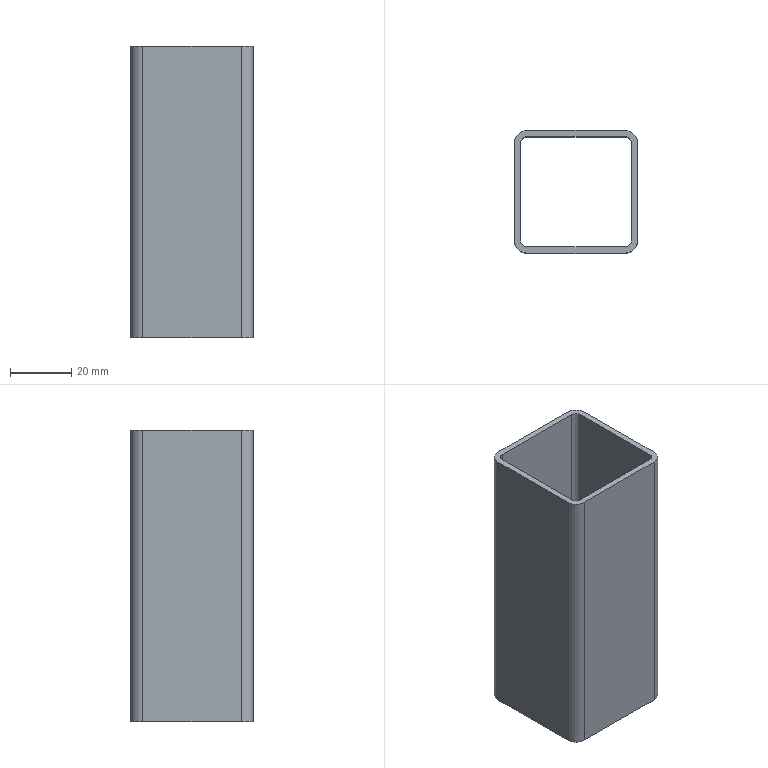Part | SolidWorks | features Fillet 2, Extrusion 1 | 1 solid | 18 faces | box 40 x 40 x 95 mm | volume 27901 mm3 | plane 10 | cylinder 8 | commonest cylinder face diameters 4 x4 8 x4
STEP:
#1=CARTESIAN_POINT('',(20.,-16.,95.));
#2=VERTEX_POINT('',#1);
#3=CARTESIAN_POINT('',(20.,16.,95.));
#4=VERTEX_POINT('',#3);
#5=CARTESIAN_POINT('',(20.,20.,95.));
#6=DIRECTION('',(0.,1.,0.));
#7=VECTOR('',#6,1000.);
#8=LINE('',#5,#7);
#9=EDGE_CURVE('',#2,#4,#8,.T.);
#10=ORIENTED_EDGE('',*,*,#9,.T.);
#11=CARTESIAN_POINT('',(16.,20.,95.));
#12=VERTEX_POINT('',#11);
#13=CARTESIAN_POINT('',(16.,16.,95.));
#14=DIRECTION('',(0.,0.,1.));
#15=DIRECTION('',(1.,0.,0.));
#16=AXIS2_PLACEMENT_3D('',#13,#14,#15);
#17=CIRCLE('',#16,4.);
#18=EDGE_CURVE('',#4,#12,#17,.T.);
#19=ORIENTED_EDGE('',*,*,#18,.T.);
#20=CARTESIAN_POINT('',(-16.,20.,95.));
#21=VERTEX_POINT('',#20);
#22=CARTESIAN_POINT('',(-20.,20.,95.));
#23=DIRECTION('',(-1.,0.,0.));
#24=VECTOR('',#23,1000.);
#25=LINE('',#22,#24);
#26=EDGE_CURVE('',#12,#21,#25,.T.);
#27=ORIENTED_EDGE('',*,*,#26,.T.);
#28=CARTESIAN_POINT('',(-20.,16.,95.));
#29=VERTEX_POINT('',#28);
#30=CARTESIAN_POINT('',(-16.,16.,95.));
#31=DIRECTION('',(0.,0.,1.));
#32=DIRECTION('',(1.,0.,0.));
#33=AXIS2_PLACEMENT_3D('',#30,#31,#32);
#34=CIRCLE('',#33,4.);
#35=EDGE_CURVE('',#21,#29,#34,.T.);
#36=ORIENTED_EDGE('',*,*,#35,.T.);
#37=CARTESIAN_POINT('',(-20.,-16.,95.));
#38=VERTEX_POINT('',#37);
#39=CARTESIAN_POINT('',(-20.,20.,95.));
#40=DIRECTION('',(0.,-1.,0.));
#41=VECTOR('',#40,1000.);
#42=LINE('',#39,#41);
#43=EDGE_CURVE('',#29,#38,#42,.T.);
#44=ORIENTED_EDGE('',*,*,#43,.T.);
#45=CARTESIAN_POINT('',(-16.,-20.,95.));
#46=VERTEX_POINT('',#45);
#47=CARTESIAN_POINT('',(-16.,-16.,95.));
#48=DIRECTION('',(0.,0.,1.));
#49=DIRECTION('',(1.,0.,0.));
#50=AXIS2_PLACEMENT_3D('',#47,#48,#49);
#51=CIRCLE('',#50,4.);
#52=EDGE_CURVE('',#38,#46,#51,.T.);
#53=ORIENTED_EDGE('',*,*,#52,.T.);
#54=CARTESIAN_POINT('',(16.,-20.,95.));
#55=VERTEX_POINT('',#54);
#56=CARTESIAN_POINT('',(-20.,-20.,95.));
#57=DIRECTION('',(1.,0.,0.));
#58=VECTOR('',#57,1000.);
#59=LINE('',#56,#58);
#60=EDGE_CURVE('',#46,#55,#59,.T.);
#61=ORIENTED_EDGE('',*,*,#60,.T.);
#62=CARTESIAN_POINT('',(16.,-16.,95.));
#63=DIRECTION('',(0.,0.,1.));
#64=DIRECTION('',(1.,0.,0.));
#65=AXIS2_PLACEMENT_3D('',#62,#63,#64);
#66=CIRCLE('',#65,4.);
#67=EDGE_CURVE('',#55,#2,#66,.T.);
#68=ORIENTED_EDGE('',*,*,#67,.T.);
#69=EDGE_LOOP('',(#10,#19,#27,#36,#44,#53,#61,#68));
#70=FACE_OUTER_BOUND('',#69,.T.);
#71=CARTESIAN_POINT('',(16.,18.,95.));
#72=VERTEX_POINT('',#71);
#73=CARTESIAN_POINT('',(-16.,18.,95.));
#74=VERTEX_POINT('',#73);
#75=CARTESIAN_POINT('',(-18.,18.,95.));
#76=DIRECTION('',(-1.,0.,0.));
#77=VECTOR('',#76,1000.);
#78=LINE('',#75,#77);
#79=EDGE_CURVE('',#72,#74,#78,.T.);
#80=ORIENTED_EDGE('',*,*,#79,.F.);
#81=CARTESIAN_POINT('',(18.,16.,95.));
#82=VERTEX_POINT('',#81);
#83=CARTESIAN_POINT('',(16.,16.,95.));
#84=DIRECTION('',(0.,0.,-1.));
#85=DIRECTION('',(1.,0.,0.));
#86=AXIS2_PLACEMENT_3D('',#83,#84,#85);
#87=CIRCLE('',#86,2.);
#88=EDGE_CURVE('',#72,#82,#87,.T.);
#89=ORIENTED_EDGE('',*,*,#88,.T.);
#90=CARTESIAN_POINT('',(18.,-16.,95.));
#91=VERTEX_POINT('',#90);
#92=CARTESIAN_POINT('',(18.,18.,95.));
#93=DIRECTION('',(0.,1.,0.));
#94=VECTOR('',#93,1000.);
#95=LINE('',#92,#94);
#96=EDGE_CURVE('',#91,#82,#95,.T.);
#97=ORIENTED_EDGE('',*,*,#96,.F.);
#98=CARTESIAN_POINT('',(16.,-18.,95.));
#99=VERTEX_POINT('',#98);
#100=CARTESIAN_POINT('',(16.,-16.,95.));
#101=DIRECTION('',(0.,0.,-1.));
#102=DIRECTION('',(1.,0.,0.));
#103=AXIS2_PLACEMENT_3D('',#100,#101,#102);
#104=CIRCLE('',#103,2.);
#105=EDGE_CURVE('',#91,#99,#104,.T.);
#106=ORIENTED_EDGE('',*,*,#105,.T.);
#107=CARTESIAN_POINT('',(-16.,-18.,95.));
#108=VERTEX_POINT('',#107);
#109=CARTESIAN_POINT('',(-18.,-18.,95.));
#110=DIRECTION('',(1.,0.,0.));
#111=VECTOR('',#110,1000.);
#112=LINE('',#109,#111);
#113=EDGE_CURVE('',#108,#99,#112,.T.);
#114=ORIENTED_EDGE('',*,*,#113,.F.);
#115=CARTESIAN_POINT('',(-18.,-16.,95.));
#116=VERTEX_POINT('',#115);
#117=CARTESIAN_POINT('',(-16.,-16.,95.));
#118=DIRECTION('',(0.,0.,-1.));
#119=DIRECTION('',(1.,0.,0.));
#120=AXIS2_PLACEMENT_3D('',#117,#118,#119);
#121=CIRCLE('',#120,2.);
#122=EDGE_CURVE('',#108,#116,#121,.T.);
#123=ORIENTED_EDGE('',*,*,#122,.T.);
#124=CARTESIAN_POINT('',(-18.,16.,95.));
#125=VERTEX_POINT('',#124);
#126=CARTESIAN_POINT('',(-18.,18.,95.));
#127=DIRECTION('',(0.,-1.,0.));
#128=VECTOR('',#127,1000.);
#129=LINE('',#126,#128);
#130=EDGE_CURVE('',#125,#116,#129,.T.);
#131=ORIENTED_EDGE('',*,*,#130,.F.);
#132=CARTESIAN_POINT('',(-16.,16.,95.));
#133=DIRECTION('',(0.,0.,-1.));
#134=DIRECTION('',(1.,0.,0.));
#135=AXIS2_PLACEMENT_3D('',#132,#133,#134);
#136=CIRCLE('',#135,2.);
#137=EDGE_CURVE('',#125,#74,#136,.T.);
#138=ORIENTED_EDGE('',*,*,#137,.T.);
#139=EDGE_LOOP('',(#80,#89,#97,#106,#114,#123,#131,#138));
#140=FACE_BOUND('',#139,.T.);
#141=CARTESIAN_POINT('',(0.,0.,95.));
#142=DIRECTION('',(0.,0.,1.));
#143=DIRECTION('',(1.,0.,0.));
#144=AXIS2_PLACEMENT_3D('',#141,#142,#143);
#145=PLANE('',#144);
#146=ADVANCED_FACE('',(#70,#140),#145,.T.);
#147=CARTESIAN_POINT('',(16.,20.,0.));
#148=VERTEX_POINT('',#147);
#149=CARTESIAN_POINT('',(-16.,20.,0.));
#150=VERTEX_POINT('',#149);
#151=CARTESIAN_POINT('',(-20.,20.,0.));
#152=DIRECTION('',(-1.,0.,0.));
#153=VECTOR('',#152,1000.);
#154=LINE('',#151,#153);
#155=EDGE_CURVE('',#148,#150,#154,.T.);
#156=ORIENTED_EDGE('',*,*,#155,.F.);
#157=CARTESIAN_POINT('',(20.,16.,0.));
#158=VERTEX_POINT('',#157);
#159=CARTESIAN_POINT('',(16.,16.,0.));
#160=DIRECTION('',(0.,0.,-1.));
#161=DIRECTION('',(1.,0.,0.));
#162=AXIS2_PLACEMENT_3D('',#159,#160,#161);
#163=CIRCLE('',#162,4.);
#164=EDGE_CURVE('',#148,#158,#163,.T.);
#165=ORIENTED_EDGE('',*,*,#164,.T.);
#166=CARTESIAN_POINT('',(20.,-16.,0.));
#167=VERTEX_POINT('',#166);
#168=CARTESIAN_POINT('',(20.,20.,0.));
#169=DIRECTION('',(0.,1.,0.));
#170=VECTOR('',#169,1000.);
#171=LINE('',#168,#170);
#172=EDGE_CURVE('',#167,#158,#171,.T.);
#173=ORIENTED_EDGE('',*,*,#172,.F.);
#174=CARTESIAN_POINT('',(16.,-20.,0.));
#175=VERTEX_POINT('',#174);
#176=CARTESIAN_POINT('',(16.,-16.,0.));
#177=DIRECTION('',(0.,0.,-1.));
#178=DIRECTION('',(1.,0.,0.));
#179=AXIS2_PLACEMENT_3D('',#176,#177,#178);
#180=CIRCLE('',#179,4.);
#181=EDGE_CURVE('',#167,#175,#180,.T.);
#182=ORIENTED_EDGE('',*,*,#181,.T.);
#183=CARTESIAN_POINT('',(-16.,-20.,0.));
#184=VERTEX_POINT('',#183);
#185=CARTESIAN_POINT('',(-20.,-20.,0.));
#186=DIRECTION('',(1.,0.,0.));
#187=VECTOR('',#186,1000.);
#188=LINE('',#185,#187);
#189=EDGE_CURVE('',#184,#175,#188,.T.);
#190=ORIENTED_EDGE('',*,*,#189,.F.);
#191=CARTESIAN_POINT('',(-20.,-16.,0.));
#192=VERTEX_POINT('',#191);
#193=CARTESIAN_POINT('',(-16.,-16.,0.));
#194=DIRECTION('',(0.,0.,-1.));
#195=DIRECTION('',(1.,0.,0.));
#196=AXIS2_PLACEMENT_3D('',#193,#194,#195);
#197=CIRCLE('',#196,4.);
#198=EDGE_CURVE('',#184,#192,#197,.T.);
#199=ORIENTED_EDGE('',*,*,#198,.T.);
#200=CARTESIAN_POINT('',(-20.,16.,0.));
#201=VERTEX_POINT('',#200);
#202=CARTESIAN_POINT('',(-20.,20.,0.));
#203=DIRECTION('',(0.,-1.,0.));
#204=VECTOR('',#203,1000.);
#205=LINE('',#202,#204);
#206=EDGE_CURVE('',#201,#192,#205,.T.);
#207=ORIENTED_EDGE('',*,*,#206,.F.);
#208=CARTESIAN_POINT('',(-16.,16.,0.));
#209=DIRECTION('',(0.,0.,-1.));
#210=DIRECTION('',(1.,0.,0.));
#211=AXIS2_PLACEMENT_3D('',#208,#209,#210);
#212=CIRCLE('',#211,4.);
#213=EDGE_CURVE('',#201,#150,#212,.T.);
#214=ORIENTED_EDGE('',*,*,#213,.T.);
#215=EDGE_LOOP('',(#156,#165,#173,#182,#190,#199,#207,#214));
#216=FACE_OUTER_BOUND('',#215,.T.);
#217=CARTESIAN_POINT('',(-16.,-18.,0.));
#218=VERTEX_POINT('',#217);
#219=CARTESIAN_POINT('',(16.,-18.,0.));
#220=VERTEX_POINT('',#219);
#221=CARTESIAN_POINT('',(-18.,-18.,0.));
#222=DIRECTION('',(1.,0.,0.));
#223=VECTOR('',#222,1000.);
#224=LINE('',#221,#223);
#225=EDGE_CURVE('',#218,#220,#224,.T.);
#226=ORIENTED_EDGE('',*,*,#225,.T.);
#227=CARTESIAN_POINT('',(18.,-16.,0.));
#228=VERTEX_POINT('',#227);
#229=CARTESIAN_POINT('',(16.,-16.,0.));
#230=DIRECTION('',(0.,0.,1.));
#231=DIRECTION('',(1.,0.,0.));
#232=AXIS2_PLACEMENT_3D('',#229,#230,#231);
#233=CIRCLE('',#232,2.);
#234=EDGE_CURVE('',#220,#228,#233,.T.);
#235=ORIENTED_EDGE('',*,*,#234,.T.);
#236=CARTESIAN_POINT('',(18.,16.,0.));
#237=VERTEX_POINT('',#236);
#238=CARTESIAN_POINT('',(18.,18.,0.));
#239=DIRECTION('',(0.,1.,0.));
#240=VECTOR('',#239,1000.);
#241=LINE('',#238,#240);
#242=EDGE_CURVE('',#228,#237,#241,.T.);
#243=ORIENTED_EDGE('',*,*,#242,.T.);
#244=CARTESIAN_POINT('',(16.,18.,0.));
#245=VERTEX_POINT('',#244);
#246=CARTESIAN_POINT('',(16.,16.,0.));
#247=DIRECTION('',(0.,0.,1.));
#248=DIRECTION('',(1.,0.,0.));
#249=AXIS2_PLACEMENT_3D('',#246,#247,#248);
#250=CIRCLE('',#249,2.);
#251=EDGE_CURVE('',#237,#245,#250,.T.);
#252=ORIENTED_EDGE('',*,*,#251,.T.);
#253=CARTESIAN_POINT('',(-16.,18.,0.));
#254=VERTEX_POINT('',#253);
#255=CARTESIAN_POINT('',(-18.,18.,0.));
#256=DIRECTION('',(-1.,0.,0.));
#257=VECTOR('',#256,1000.);
#258=LINE('',#255,#257);
#259=EDGE_CURVE('',#245,#254,#258,.T.);
#260=ORIENTED_EDGE('',*,*,#259,.T.);
#261=CARTESIAN_POINT('',(-18.,16.,0.));
#262=VERTEX_POINT('',#261);
#263=CARTESIAN_POINT('',(-16.,16.,0.));
#264=DIRECTION('',(0.,0.,1.));
#265=DIRECTION('',(1.,0.,0.));
#266=AXIS2_PLACEMENT_3D('',#263,#264,#265);
#267=CIRCLE('',#266,2.);
#268=EDGE_CURVE('',#254,#262,#267,.T.);
#269=ORIENTED_EDGE('',*,*,#268,.T.);
#270=CARTESIAN_POINT('',(-18.,-16.,0.));
#271=VERTEX_POINT('',#270);
#272=CARTESIAN_POINT('',(-18.,18.,0.));
#273=DIRECTION('',(0.,-1.,0.));
#274=VECTOR('',#273,1000.);
#275=LINE('',#272,#274);
#276=EDGE_CURVE('',#262,#271,#275,.T.);
#277=ORIENTED_EDGE('',*,*,#276,.T.);
#278=CARTESIAN_POINT('',(-16.,-16.,0.));
#279=DIRECTION('',(0.,0.,1.));
#280=DIRECTION('',(1.,0.,0.));
#281=AXIS2_PLACEMENT_3D('',#278,#279,#280);
#282=CIRCLE('',#281,2.);
#283=EDGE_CURVE('',#271,#218,#282,.T.);
#284=ORIENTED_EDGE('',*,*,#283,.T.);
#285=EDGE_LOOP('',(#226,#235,#243,#252,#260,#269,#277,#284));
#286=FACE_BOUND('',#285,.T.);
#287=CARTESIAN_POINT('',(0.,0.,0.));
#288=DIRECTION('',(0.,0.,1.));
#289=DIRECTION('',(1.,0.,0.));
#290=AXIS2_PLACEMENT_3D('',#287,#288,#289);
#291=PLANE('',#290);
#292=ADVANCED_FACE('',(#216,#286),#291,.F.);
#293=ORIENTED_EDGE('',*,*,#172,.T.);
#294=CARTESIAN_POINT('',(20.,16.,95.));
#295=DIRECTION('',(0.,0.,1.));
#296=VECTOR('',#295,1000.);
#297=LINE('',#294,#296);
#298=EDGE_CURVE('',#158,#4,#297,.T.);
#299=ORIENTED_EDGE('',*,*,#298,.T.);
#300=ORIENTED_EDGE('',*,*,#9,.F.);
#301=CARTESIAN_POINT('',(20.,-16.,95.));
#302=DIRECTION('',(0.,0.,-1.));
#303=VECTOR('',#302,1000.);
#304=LINE('',#301,#303);
#305=EDGE_CURVE('',#2,#167,#304,.T.);
#306=ORIENTED_EDGE('',*,*,#305,.T.);
#307=EDGE_LOOP('',(#293,#299,#300,#306));
#308=FACE_OUTER_BOUND('',#307,.T.);
#309=CARTESIAN_POINT('',(20.,20.,95.));
#310=DIRECTION('',(-1.,0.,0.));
#311=DIRECTION('',(0.,0.,1.));
#312=AXIS2_PLACEMENT_3D('',#309,#310,#311);
#313=PLANE('',#312);
#314=ADVANCED_FACE('',(#308),#313,.F.);
#315=ORIENTED_EDGE('',*,*,#26,.F.);
#316=CARTESIAN_POINT('',(16.,20.,95.));
#317=DIRECTION('',(0.,0.,-1.));
#318=VECTOR('',#317,1000.);
#319=LINE('',#316,#318);
#320=EDGE_CURVE('',#12,#148,#319,.T.);
#321=ORIENTED_EDGE('',*,*,#320,.T.);
#322=ORIENTED_EDGE('',*,*,#155,.T.);
#323=CARTESIAN_POINT('',(-16.,20.,95.));
#324=DIRECTION('',(0.,0.,1.));
#325=VECTOR('',#324,1000.);
#326=LINE('',#323,#325);
#327=EDGE_CURVE('',#150,#21,#326,.T.);
#328=ORIENTED_EDGE('',*,*,#327,.T.);
#329=EDGE_LOOP('',(#315,#321,#322,#328));
#330=FACE_OUTER_BOUND('',#329,.T.);
#331=CARTESIAN_POINT('',(-20.,20.,95.));
#332=DIRECTION('',(0.,-1.,0.));
#333=DIRECTION('',(0.,0.,-1.));
#334=AXIS2_PLACEMENT_3D('',#331,#332,#333);
#335=PLANE('',#334);
#336=ADVANCED_FACE('',(#330),#335,.F.);
#337=ORIENTED_EDGE('',*,*,#43,.F.);
#338=CARTESIAN_POINT('',(-20.,16.,95.));
#339=DIRECTION('',(0.,0.,-1.));
#340=VECTOR('',#339,1000.);
#341=LINE('',#338,#340);
#342=EDGE_CURVE('',#29,#201,#341,.T.);
#343=ORIENTED_EDGE('',*,*,#342,.T.);
#344=ORIENTED_EDGE('',*,*,#206,.T.);
#345=CARTESIAN_POINT('',(-20.,-16.,95.));
#346=DIRECTION('',(0.,0.,1.));
#347=VECTOR('',#346,1000.);
#348=LINE('',#345,#347);
#349=EDGE_CURVE('',#192,#38,#348,.T.);
#350=ORIENTED_EDGE('',*,*,#349,.T.);
#351=EDGE_LOOP('',(#337,#343,#344,#350));
#352=FACE_OUTER_BOUND('',#351,.T.);
#353=CARTESIAN_POINT('',(-20.,20.,95.));
#354=DIRECTION('',(1.,0.,0.));
#355=DIRECTION('',(0.,0.,-1.));
#356=AXIS2_PLACEMENT_3D('',#353,#354,#355);
#357=PLANE('',#356);
#358=ADVANCED_FACE('',(#352),#357,.F.);
#359=ORIENTED_EDGE('',*,*,#189,.T.);
#360=CARTESIAN_POINT('',(16.,-20.,95.));
#361=DIRECTION('',(0.,0.,1.));
#362=VECTOR('',#361,1000.);
#363=LINE('',#360,#362);
#364=EDGE_CURVE('',#175,#55,#363,.T.);
#365=ORIENTED_EDGE('',*,*,#364,.T.);
#366=ORIENTED_EDGE('',*,*,#60,.F.);
#367=CARTESIAN_POINT('',(-16.,-20.,95.));
#368=DIRECTION('',(0.,0.,-1.));
#369=VECTOR('',#368,1000.);
#370=LINE('',#367,#369);
#371=EDGE_CURVE('',#46,#184,#370,.T.);
#372=ORIENTED_EDGE('',*,*,#371,.T.);
#373=EDGE_LOOP('',(#359,#365,#366,#372));
#374=FACE_OUTER_BOUND('',#373,.T.);
#375=CARTESIAN_POINT('',(-20.,-20.,95.));
#376=DIRECTION('',(0.,1.,0.));
#377=DIRECTION('',(0.,0.,1.));
#378=AXIS2_PLACEMENT_3D('',#375,#376,#377);
#379=PLANE('',#378);
#380=ADVANCED_FACE('',(#374),#379,.F.);
#381=ORIENTED_EDGE('',*,*,#96,.T.);
#382=CARTESIAN_POINT('',(18.,16.,0.));
#383=DIRECTION('',(0.,0.,-1.));
#384=VECTOR('',#383,1000.);
#385=LINE('',#382,#384);
#386=EDGE_CURVE('',#82,#237,#385,.T.);
#387=ORIENTED_EDGE('',*,*,#386,.T.);
#388=ORIENTED_EDGE('',*,*,#242,.F.);
#389=CARTESIAN_POINT('',(18.,-16.,95.));
#390=DIRECTION('',(0.,0.,1.));
#391=VECTOR('',#390,1000.);
#392=LINE('',#389,#391);
#393=EDGE_CURVE('',#228,#91,#392,.T.);
#394=ORIENTED_EDGE('',*,*,#393,.T.);
#395=EDGE_LOOP('',(#381,#387,#388,#394));
#396=FACE_OUTER_BOUND('',#395,.T.);
#397=CARTESIAN_POINT('',(18.,18.,95.));
#398=DIRECTION('',(-1.,0.,0.));
#399=DIRECTION('',(0.,0.,1.));
#400=AXIS2_PLACEMENT_3D('',#397,#398,#399);
#401=PLANE('',#400);
#402=ADVANCED_FACE('',(#396),#401,.T.);
#403=ORIENTED_EDGE('',*,*,#259,.F.);
#404=CARTESIAN_POINT('',(16.,18.,95.));
#405=DIRECTION('',(0.,0.,1.));
#406=VECTOR('',#405,1000.);
#407=LINE('',#404,#406);
#408=EDGE_CURVE('',#245,#72,#407,.T.);
#409=ORIENTED_EDGE('',*,*,#408,.T.);
#410=ORIENTED_EDGE('',*,*,#79,.T.);
#411=CARTESIAN_POINT('',(-16.,18.,0.));
#412=DIRECTION('',(0.,0.,-1.));
#413=VECTOR('',#412,1000.);
#414=LINE('',#411,#413);
#415=EDGE_CURVE('',#74,#254,#414,.T.);
#416=ORIENTED_EDGE('',*,*,#415,.T.);
#417=EDGE_LOOP('',(#403,#409,#410,#416));
#418=FACE_OUTER_BOUND('',#417,.T.);
#419=CARTESIAN_POINT('',(-18.,18.,95.));
#420=DIRECTION('',(0.,-1.,0.));
#421=DIRECTION('',(0.,0.,-1.));
#422=AXIS2_PLACEMENT_3D('',#419,#420,#421);
#423=PLANE('',#422);
#424=ADVANCED_FACE('',(#418),#423,.T.);
#425=ORIENTED_EDGE('',*,*,#276,.F.);
#426=CARTESIAN_POINT('',(-18.,16.,95.));
#427=DIRECTION('',(0.,0.,1.));
#428=VECTOR('',#427,1000.);
#429=LINE('',#426,#428);
#430=EDGE_CURVE('',#262,#125,#429,.T.);
#431=ORIENTED_EDGE('',*,*,#430,.T.);
#432=ORIENTED_EDGE('',*,*,#130,.T.);
#433=CARTESIAN_POINT('',(-18.,-16.,0.));
#434=DIRECTION('',(0.,0.,-1.));
#435=VECTOR('',#434,1000.);
#436=LINE('',#433,#435);
#437=EDGE_CURVE('',#116,#271,#436,.T.);
#438=ORIENTED_EDGE('',*,*,#437,.T.);
#439=EDGE_LOOP('',(#425,#431,#432,#438));
#440=FACE_OUTER_BOUND('',#439,.T.);
#441=CARTESIAN_POINT('',(-18.,18.,95.));
#442=DIRECTION('',(1.,0.,0.));
#443=DIRECTION('',(0.,0.,-1.));
#444=AXIS2_PLACEMENT_3D('',#441,#442,#443);
#445=PLANE('',#444);
#446=ADVANCED_FACE('',(#440),#445,.T.);
#447=ORIENTED_EDGE('',*,*,#225,.F.);
#448=CARTESIAN_POINT('',(-16.,-18.,95.));
#449=DIRECTION('',(0.,0.,1.));
#450=VECTOR('',#449,1000.);
#451=LINE('',#448,#450);
#452=EDGE_CURVE('',#218,#108,#451,.T.);
#453=ORIENTED_EDGE('',*,*,#452,.T.);
#454=ORIENTED_EDGE('',*,*,#113,.T.);
#455=CARTESIAN_POINT('',(16.,-18.,0.));
#456=DIRECTION('',(0.,0.,-1.));
#457=VECTOR('',#456,1000.);
#458=LINE('',#455,#457);
#459=EDGE_CURVE('',#99,#220,#458,.T.);
#460=ORIENTED_EDGE('',*,*,#459,.T.);
#461=EDGE_LOOP('',(#447,#453,#454,#460));
#462=FACE_OUTER_BOUND('',#461,.T.);
#463=CARTESIAN_POINT('',(-18.,-18.,95.));
#464=DIRECTION('',(0.,1.,0.));
#465=DIRECTION('',(0.,0.,1.));
#466=AXIS2_PLACEMENT_3D('',#463,#464,#465);
#467=PLANE('',#466);
#468=ADVANCED_FACE('',(#462),#467,.T.);
#469=ORIENTED_EDGE('',*,*,#88,.F.);
#470=ORIENTED_EDGE('',*,*,#408,.F.);
#471=ORIENTED_EDGE('',*,*,#251,.F.);
#472=ORIENTED_EDGE('',*,*,#386,.F.);
#473=EDGE_LOOP('',(#469,#470,#471,#472));
#474=FACE_OUTER_BOUND('',#473,.T.);
#475=CARTESIAN_POINT('',(16.,16.,95.));
#476=DIRECTION('',(0.,0.,1.));
#477=DIRECTION('',(1.,0.,0.));
#478=AXIS2_PLACEMENT_3D('',#475,#476,#477);
#479=CYLINDRICAL_SURFACE('',#478,2.);
#480=ADVANCED_FACE('',(#474),#479,.F.);
#481=ORIENTED_EDGE('',*,*,#137,.F.);
#482=ORIENTED_EDGE('',*,*,#430,.F.);
#483=ORIENTED_EDGE('',*,*,#268,.F.);
#484=ORIENTED_EDGE('',*,*,#415,.F.);
#485=EDGE_LOOP('',(#481,#482,#483,#484));
#486=FACE_OUTER_BOUND('',#485,.T.);
#487=CARTESIAN_POINT('',(-16.,16.,95.));
#488=DIRECTION('',(0.,0.,1.));
#489=DIRECTION('',(1.,0.,0.));
#490=AXIS2_PLACEMENT_3D('',#487,#488,#489);
#491=CYLINDRICAL_SURFACE('',#490,2.);
#492=ADVANCED_FACE('',(#486),#491,.F.);
#493=ORIENTED_EDGE('',*,*,#122,.F.);
#494=ORIENTED_EDGE('',*,*,#452,.F.);
#495=ORIENTED_EDGE('',*,*,#283,.F.);
#496=ORIENTED_EDGE('',*,*,#437,.F.);
#497=EDGE_LOOP('',(#493,#494,#495,#496));
#498=FACE_OUTER_BOUND('',#497,.T.);
#499=CARTESIAN_POINT('',(-16.,-16.,95.));
#500=DIRECTION('',(0.,0.,1.));
#501=DIRECTION('',(1.,0.,0.));
#502=AXIS2_PLACEMENT_3D('',#499,#500,#501);
#503=CYLINDRICAL_SURFACE('',#502,2.);
#504=ADVANCED_FACE('',(#498),#503,.F.);
#505=ORIENTED_EDGE('',*,*,#105,.F.);
#506=ORIENTED_EDGE('',*,*,#393,.F.);
#507=ORIENTED_EDGE('',*,*,#234,.F.);
#508=ORIENTED_EDGE('',*,*,#459,.F.);
#509=EDGE_LOOP('',(#505,#506,#507,#508));
#510=FACE_OUTER_BOUND('',#509,.T.);
#511=CARTESIAN_POINT('',(16.,-16.,95.));
#512=DIRECTION('',(0.,0.,1.));
#513=DIRECTION('',(1.,0.,0.));
#514=AXIS2_PLACEMENT_3D('',#511,#512,#513);
#515=CYLINDRICAL_SURFACE('',#514,2.);
#516=ADVANCED_FACE('',(#510),#515,.F.);
#517=ORIENTED_EDGE('',*,*,#18,.F.);
#518=ORIENTED_EDGE('',*,*,#298,.F.);
#519=ORIENTED_EDGE('',*,*,#164,.F.);
#520=ORIENTED_EDGE('',*,*,#320,.F.);
#521=EDGE_LOOP('',(#517,#518,#519,#520));
#522=FACE_OUTER_BOUND('',#521,.T.);
#523=CARTESIAN_POINT('',(16.,16.,95.));
#524=DIRECTION('',(0.,0.,-1.));
#525=DIRECTION('',(-1.,0.,0.));
#526=AXIS2_PLACEMENT_3D('',#523,#524,#525);
#527=CYLINDRICAL_SURFACE('',#526,4.);
#528=ADVANCED_FACE('',(#522),#527,.T.);
#529=ORIENTED_EDGE('',*,*,#67,.F.);
#530=ORIENTED_EDGE('',*,*,#364,.F.);
#531=ORIENTED_EDGE('',*,*,#181,.F.);
#532=ORIENTED_EDGE('',*,*,#305,.F.);
#533=EDGE_LOOP('',(#529,#530,#531,#532));
#534=FACE_OUTER_BOUND('',#533,.T.);
#535=CARTESIAN_POINT('',(16.,-16.,95.));
#536=DIRECTION('',(0.,0.,-1.));
#537=DIRECTION('',(-1.,0.,0.));
#538=AXIS2_PLACEMENT_3D('',#535,#536,#537);
#539=CYLINDRICAL_SURFACE('',#538,4.);
#540=ADVANCED_FACE('',(#534),#539,.T.);
#541=ORIENTED_EDGE('',*,*,#35,.F.);
#542=ORIENTED_EDGE('',*,*,#327,.F.);
#543=ORIENTED_EDGE('',*,*,#213,.F.);
#544=ORIENTED_EDGE('',*,*,#342,.F.);
#545=EDGE_LOOP('',(#541,#542,#543,#544));
#546=FACE_OUTER_BOUND('',#545,.T.);
#547=CARTESIAN_POINT('',(-16.,16.,95.));
#548=DIRECTION('',(0.,0.,-1.));
#549=DIRECTION('',(-1.,0.,0.));
#550=AXIS2_PLACEMENT_3D('',#547,#548,#549);
#551=CYLINDRICAL_SURFACE('',#550,4.);
#552=ADVANCED_FACE('',(#546),#551,.T.);
#553=ORIENTED_EDGE('',*,*,#52,.F.);
#554=ORIENTED_EDGE('',*,*,#349,.F.);
#555=ORIENTED_EDGE('',*,*,#198,.F.);
#556=ORIENTED_EDGE('',*,*,#371,.F.);
#557=EDGE_LOOP('',(#553,#554,#555,#556));
#558=FACE_OUTER_BOUND('',#557,.T.);
#559=CARTESIAN_POINT('',(-16.,-16.,95.));
#560=DIRECTION('',(0.,0.,-1.));
#561=DIRECTION('',(-1.,0.,0.));
#562=AXIS2_PLACEMENT_3D('',#559,#560,#561);
#563=CYLINDRICAL_SURFACE('',#562,4.);
#564=ADVANCED_FACE('',(#558),#563,.T.);
#565=CLOSED_SHELL('',(#146,#292,#314,#336,#358,#380,#402,#424,#446,#468,#480,#492,#504,#516,#528,#540,#552,#564));
#566=MANIFOLD_SOLID_BREP('',#565);
#567=CARTESIAN_POINT('',(0.,0.,0.));
#568=DIRECTION('',(0.,0.,1.));
#569=DIRECTION('',(1.,0.,0.));
#570=AXIS2_PLACEMENT_3D('',#567,#568,#569);
#571=(LENGTH_UNIT()NAMED_UNIT(*)SI_UNIT(.MILLI.,.METRE.));
#572=UNCERTAINTY_MEASURE_WITH_UNIT(LENGTH_MEASURE(0.00001),#571,'','');
#573=(NAMED_UNIT(*)PLANE_ANGLE_UNIT()SI_UNIT($,.RADIAN.));
#574=(NAMED_UNIT(*)SI_UNIT($,.STERADIAN.)SOLID_ANGLE_UNIT());
#575=(GEOMETRIC_REPRESENTATION_CONTEXT(3)GLOBAL_UNCERTAINTY_ASSIGNED_CONTEXT((#572))GLOBAL_UNIT_ASSIGNED_CONTEXT((#571,#573,#574))REPRESENTATION_CONTEXT('',''));
#576=ADVANCED_BREP_SHAPE_REPRESENTATION('',(#566,#570),#575);